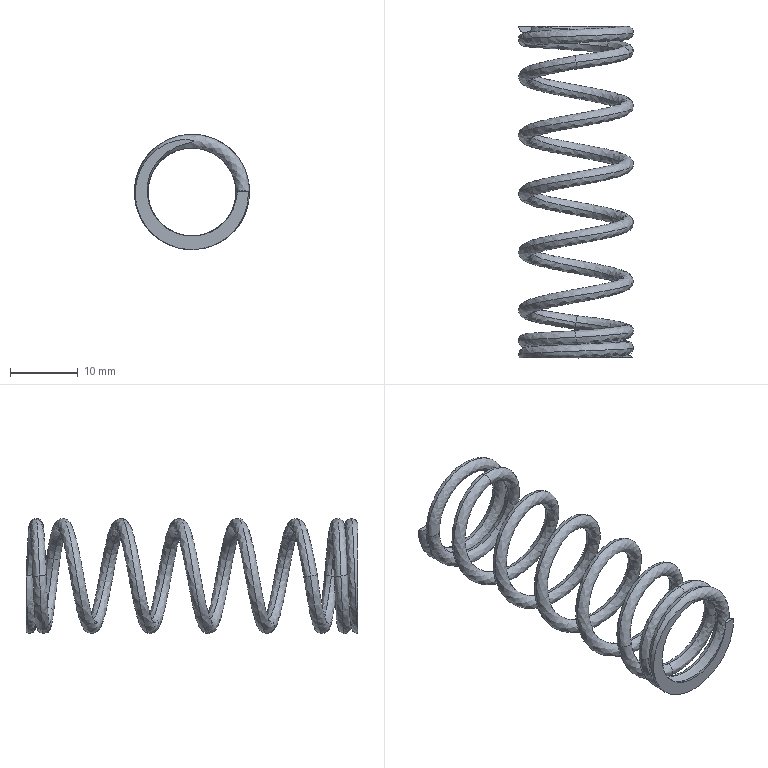Part | STEP file | Compression spring 1_1 | 1 solid | 26 faces | volume 1226 mm3 | spline 22 | plane 4